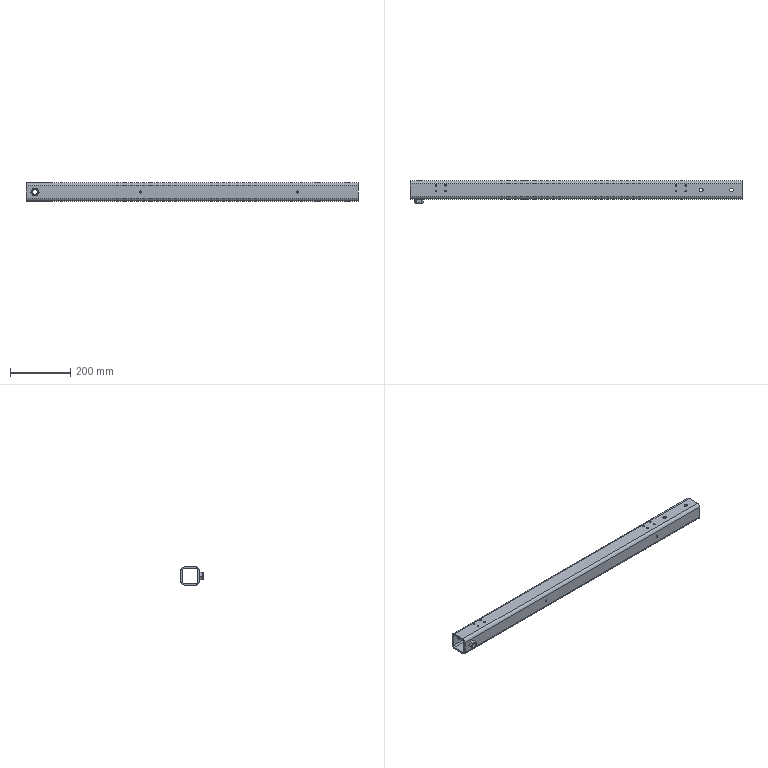Part | 2 solids | 98 faces | box 1100 x 73 x 60 mm | volume 1135660 mm3 | cylinder 66 | plane 26 | cone 6 | commonest cylinder face diameters 5 x32 6.8 x8 12 x8 10 x4 19 x4 20 x4